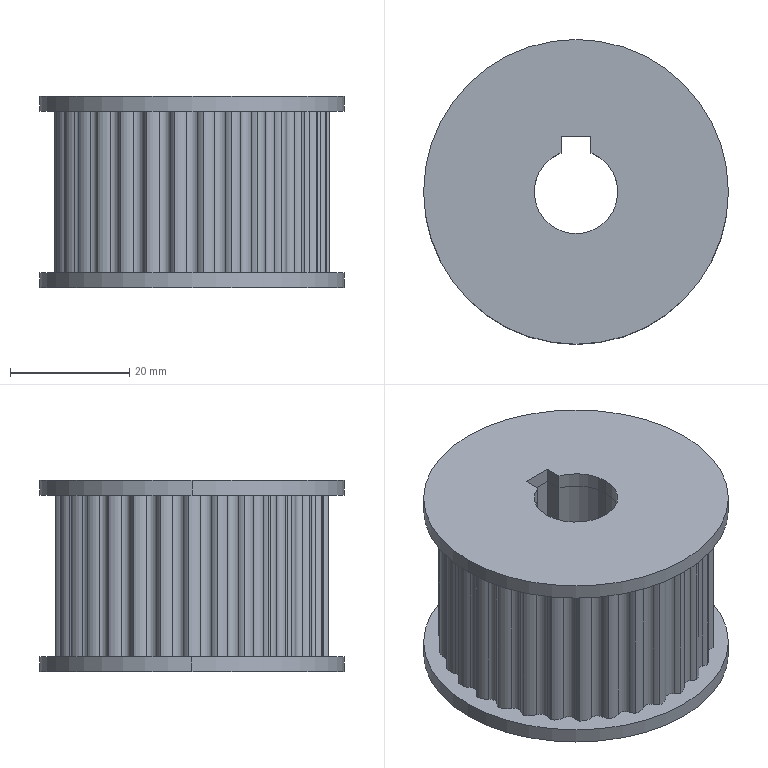Part | 2 solids | 130 faces | box 51 x 51 x 32 mm | volume 47147 mm3 | cylinder 118 | plane 12 | commonest cylinder face diameters 5 x69 2.5 x39 14 x6 51 x4